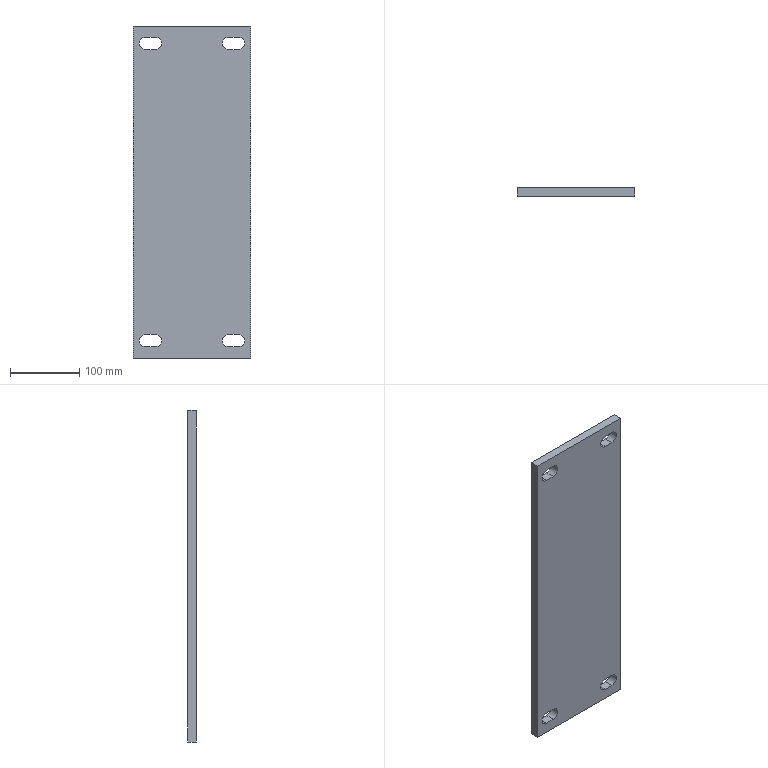Part | SolidWorks | features BaseBody 1 | 1 solid | 22 faces | box 170 x 13 x 480 mm | volume 1034464 mm3 | plane 14 | cylinder 8 | commonest cylinder face diameters 18 x8
STEP:
#1=CARTESIAN_POINT('',(-10.701,8.606,34.));
#2=VERTEX_POINT('',#1);
#3=CARTESIAN_POINT('',(-10.701,8.606,16.));
#4=VERTEX_POINT('',#3);
#5=CARTESIAN_POINT('',(-10.701,8.606,25.));
#6=DIRECTION('',(0.,-1.,0.));
#7=DIRECTION('',(0.,0.,-1.));
#8=AXIS2_PLACEMENT_3D('',#5,#6,#7);
#9=CIRCLE('',#8,9.);
#10=EDGE_CURVE('',#2,#4,#9,.T.);
#11=ORIENTED_EDGE('',*,*,#10,.T.);
#12=CARTESIAN_POINT('',(3.299,8.606,16.));
#13=VERTEX_POINT('',#12);
#14=CARTESIAN_POINT('',(-28.701,8.606,16.));
#15=DIRECTION('',(1.,0.,0.));
#16=VECTOR('',#15,1000.);
#17=LINE('',#14,#16);
#18=EDGE_CURVE('',#4,#13,#17,.T.);
#19=ORIENTED_EDGE('',*,*,#18,.T.);
#20=CARTESIAN_POINT('',(3.299,8.606,34.));
#21=VERTEX_POINT('',#20);
#22=CARTESIAN_POINT('',(3.299,8.606,25.));
#23=DIRECTION('',(0.,-1.,0.));
#24=DIRECTION('',(0.,0.,-1.));
#25=AXIS2_PLACEMENT_3D('',#22,#23,#24);
#26=CIRCLE('',#25,9.);
#27=EDGE_CURVE('',#13,#21,#26,.T.);
#28=ORIENTED_EDGE('',*,*,#27,.T.);
#29=CARTESIAN_POINT('',(-28.701,8.606,34.));
#30=DIRECTION('',(-1.,0.,0.));
#31=VECTOR('',#30,1000.);
#32=LINE('',#29,#31);
#33=EDGE_CURVE('',#21,#2,#32,.T.);
#34=ORIENTED_EDGE('',*,*,#33,.T.);
#35=EDGE_LOOP('',(#11,#19,#28,#34));
#36=FACE_BOUND('',#35,.T.);
#37=CARTESIAN_POINT('',(-10.701,8.606,446.));
#38=VERTEX_POINT('',#37);
#39=CARTESIAN_POINT('',(3.299,8.606,446.));
#40=VERTEX_POINT('',#39);
#41=CARTESIAN_POINT('',(-28.701,8.606,446.));
#42=DIRECTION('',(1.,0.,0.));
#43=VECTOR('',#42,1000.);
#44=LINE('',#41,#43);
#45=EDGE_CURVE('',#38,#40,#44,.T.);
#46=ORIENTED_EDGE('',*,*,#45,.T.);
#47=CARTESIAN_POINT('',(3.299,8.606,464.));
#48=VERTEX_POINT('',#47);
#49=CARTESIAN_POINT('',(3.299,8.606,455.));
#50=DIRECTION('',(0.,-1.,0.));
#51=DIRECTION('',(0.,0.,-1.));
#52=AXIS2_PLACEMENT_3D('',#49,#50,#51);
#53=CIRCLE('',#52,9.);
#54=EDGE_CURVE('',#40,#48,#53,.T.);
#55=ORIENTED_EDGE('',*,*,#54,.T.);
#56=CARTESIAN_POINT('',(-10.701,8.606,464.));
#57=VERTEX_POINT('',#56);
#58=CARTESIAN_POINT('',(-28.701,8.606,464.));
#59=DIRECTION('',(-1.,0.,0.));
#60=VECTOR('',#59,1000.);
#61=LINE('',#58,#60);
#62=EDGE_CURVE('',#48,#57,#61,.T.);
#63=ORIENTED_EDGE('',*,*,#62,.T.);
#64=CARTESIAN_POINT('',(-10.701,8.606,455.));
#65=DIRECTION('',(0.,-1.,0.));
#66=DIRECTION('',(0.,0.,-1.));
#67=AXIS2_PLACEMENT_3D('',#64,#65,#66);
#68=CIRCLE('',#67,9.);
#69=EDGE_CURVE('',#57,#38,#68,.T.);
#70=ORIENTED_EDGE('',*,*,#69,.T.);
#71=EDGE_LOOP('',(#46,#55,#63,#70));
#72=FACE_BOUND('',#71,.T.);
#73=CARTESIAN_POINT('',(109.299,8.606,16.));
#74=VERTEX_POINT('',#73);
#75=CARTESIAN_POINT('',(123.299,8.606,16.));
#76=VERTEX_POINT('',#75);
#77=CARTESIAN_POINT('',(-28.701,8.606,16.));
#78=DIRECTION('',(1.,0.,0.));
#79=VECTOR('',#78,1000.);
#80=LINE('',#77,#79);
#81=EDGE_CURVE('',#74,#76,#80,.T.);
#82=ORIENTED_EDGE('',*,*,#81,.T.);
#83=CARTESIAN_POINT('',(123.299,8.606,34.));
#84=VERTEX_POINT('',#83);
#85=CARTESIAN_POINT('',(123.299,8.606,25.));
#86=DIRECTION('',(0.,-1.,0.));
#87=DIRECTION('',(0.,0.,-1.));
#88=AXIS2_PLACEMENT_3D('',#85,#86,#87);
#89=CIRCLE('',#88,9.);
#90=EDGE_CURVE('',#76,#84,#89,.T.);
#91=ORIENTED_EDGE('',*,*,#90,.T.);
#92=CARTESIAN_POINT('',(109.299,8.606,34.));
#93=VERTEX_POINT('',#92);
#94=CARTESIAN_POINT('',(-28.701,8.606,34.));
#95=DIRECTION('',(-1.,0.,0.));
#96=VECTOR('',#95,1000.);
#97=LINE('',#94,#96);
#98=EDGE_CURVE('',#84,#93,#97,.T.);
#99=ORIENTED_EDGE('',*,*,#98,.T.);
#100=CARTESIAN_POINT('',(109.299,8.606,25.));
#101=DIRECTION('',(0.,-1.,0.));
#102=DIRECTION('',(0.,0.,-1.));
#103=AXIS2_PLACEMENT_3D('',#100,#101,#102);
#104=CIRCLE('',#103,9.);
#105=EDGE_CURVE('',#93,#74,#104,.T.);
#106=ORIENTED_EDGE('',*,*,#105,.T.);
#107=EDGE_LOOP('',(#82,#91,#99,#106));
#108=FACE_BOUND('',#107,.T.);
#109=CARTESIAN_POINT('',(109.299,8.606,446.));
#110=VERTEX_POINT('',#109);
#111=CARTESIAN_POINT('',(123.299,8.606,446.));
#112=VERTEX_POINT('',#111);
#113=CARTESIAN_POINT('',(-28.701,8.606,446.));
#114=DIRECTION('',(1.,0.,0.));
#115=VECTOR('',#114,1000.);
#116=LINE('',#113,#115);
#117=EDGE_CURVE('',#110,#112,#116,.T.);
#118=ORIENTED_EDGE('',*,*,#117,.T.);
#119=CARTESIAN_POINT('',(123.299,8.606,464.));
#120=VERTEX_POINT('',#119);
#121=CARTESIAN_POINT('',(123.299,8.606,455.));
#122=DIRECTION('',(0.,-1.,0.));
#123=DIRECTION('',(0.,0.,-1.));
#124=AXIS2_PLACEMENT_3D('',#121,#122,#123);
#125=CIRCLE('',#124,9.);
#126=EDGE_CURVE('',#112,#120,#125,.T.);
#127=ORIENTED_EDGE('',*,*,#126,.T.);
#128=CARTESIAN_POINT('',(109.299,8.606,464.));
#129=VERTEX_POINT('',#128);
#130=CARTESIAN_POINT('',(-28.701,8.606,464.));
#131=DIRECTION('',(-1.,0.,0.));
#132=VECTOR('',#131,1000.);
#133=LINE('',#130,#132);
#134=EDGE_CURVE('',#120,#129,#133,.T.);
#135=ORIENTED_EDGE('',*,*,#134,.T.);
#136=CARTESIAN_POINT('',(109.299,8.606,455.));
#137=DIRECTION('',(0.,-1.,0.));
#138=DIRECTION('',(0.,0.,-1.));
#139=AXIS2_PLACEMENT_3D('',#136,#137,#138);
#140=CIRCLE('',#139,9.);
#141=EDGE_CURVE('',#129,#110,#140,.T.);
#142=ORIENTED_EDGE('',*,*,#141,.T.);
#143=EDGE_LOOP('',(#118,#127,#135,#142));
#144=FACE_BOUND('',#143,.T.);
#145=CARTESIAN_POINT('',(141.299,8.606,0.));
#146=VERTEX_POINT('',#145);
#147=CARTESIAN_POINT('',(-28.701,8.606,0.));
#148=VERTEX_POINT('',#147);
#149=CARTESIAN_POINT('',(-28.701,8.606,0.));
#150=DIRECTION('',(-1.,0.,0.));
#151=VECTOR('',#150,1000.);
#152=LINE('',#149,#151);
#153=EDGE_CURVE('',#146,#148,#152,.T.);
#154=ORIENTED_EDGE('',*,*,#153,.T.);
#155=CARTESIAN_POINT('',(-28.701,8.606,480.));
#156=VERTEX_POINT('',#155);
#157=CARTESIAN_POINT('',(-28.701,8.606,0.));
#158=DIRECTION('',(0.,0.,1.));
#159=VECTOR('',#158,1000.);
#160=LINE('',#157,#159);
#161=EDGE_CURVE('',#148,#156,#160,.T.);
#162=ORIENTED_EDGE('',*,*,#161,.T.);
#163=CARTESIAN_POINT('',(141.299,8.606,480.));
#164=VERTEX_POINT('',#163);
#165=CARTESIAN_POINT('',(-28.701,8.606,480.));
#166=DIRECTION('',(1.,0.,0.));
#167=VECTOR('',#166,1000.);
#168=LINE('',#165,#167);
#169=EDGE_CURVE('',#156,#164,#168,.T.);
#170=ORIENTED_EDGE('',*,*,#169,.T.);
#171=CARTESIAN_POINT('',(141.299,8.606,0.));
#172=DIRECTION('',(0.,0.,-1.));
#173=VECTOR('',#172,1000.);
#174=LINE('',#171,#173);
#175=EDGE_CURVE('',#164,#146,#174,.T.);
#176=ORIENTED_EDGE('',*,*,#175,.T.);
#177=EDGE_LOOP('',(#154,#162,#170,#176));
#178=FACE_OUTER_BOUND('',#177,.T.);
#179=CARTESIAN_POINT('',(-28.701,8.606,0.));
#180=DIRECTION('',(0.,1.,0.));
#181=DIRECTION('',(0.,0.,1.));
#182=AXIS2_PLACEMENT_3D('',#179,#180,#181);
#183=PLANE('',#182);
#184=ADVANCED_FACE('',(#36,#72,#108,#144,#178),#183,.T.);
#185=CARTESIAN_POINT('',(3.299,-4.394,16.));
#186=VERTEX_POINT('',#185);
#187=CARTESIAN_POINT('',(3.299,8.606,16.));
#188=DIRECTION('',(0.,-1.,0.));
#189=VECTOR('',#188,1000.);
#190=LINE('',#187,#189);
#191=EDGE_CURVE('',#13,#186,#190,.T.);
#192=ORIENTED_EDGE('',*,*,#191,.F.);
#193=ORIENTED_EDGE('',*,*,#18,.F.);
#194=CARTESIAN_POINT('',(-10.701,-4.394,16.));
#195=VERTEX_POINT('',#194);
#196=CARTESIAN_POINT('',(-10.701,8.606,16.));
#197=DIRECTION('',(0.,1.,0.));
#198=VECTOR('',#197,1000.);
#199=LINE('',#196,#198);
#200=EDGE_CURVE('',#195,#4,#199,.T.);
#201=ORIENTED_EDGE('',*,*,#200,.F.);
#202=CARTESIAN_POINT('',(3.299,-4.394,16.));
#203=DIRECTION('',(-1.,0.,0.));
#204=VECTOR('',#203,1000.);
#205=LINE('',#202,#204);
#206=EDGE_CURVE('',#186,#195,#205,.T.);
#207=ORIENTED_EDGE('',*,*,#206,.F.);
#208=EDGE_LOOP('',(#192,#193,#201,#207));
#209=FACE_OUTER_BOUND('',#208,.T.);
#210=CARTESIAN_POINT('',(3.299,8.606,16.));
#211=DIRECTION('',(0.,0.,-1.));
#212=DIRECTION('',(-1.,0.,0.));
#213=AXIS2_PLACEMENT_3D('',#210,#211,#212);
#214=PLANE('',#213);
#215=ADVANCED_FACE('',(#209),#214,.F.);
#216=ORIENTED_EDGE('',*,*,#200,.T.);
#217=ORIENTED_EDGE('',*,*,#10,.F.);
#218=CARTESIAN_POINT('',(-10.701,-4.394,34.));
#219=VERTEX_POINT('',#218);
#220=CARTESIAN_POINT('',(-10.701,8.606,34.));
#221=DIRECTION('',(0.,1.,0.));
#222=VECTOR('',#221,1000.);
#223=LINE('',#220,#222);
#224=EDGE_CURVE('',#219,#2,#223,.T.);
#225=ORIENTED_EDGE('',*,*,#224,.F.);
#226=CARTESIAN_POINT('',(-10.701,-4.394,25.));
#227=DIRECTION('',(0.,1.,0.));
#228=DIRECTION('',(0.,0.,-1.));
#229=AXIS2_PLACEMENT_3D('',#226,#227,#228);
#230=CIRCLE('',#229,9.);
#231=EDGE_CURVE('',#195,#219,#230,.T.);
#232=ORIENTED_EDGE('',*,*,#231,.F.);
#233=EDGE_LOOP('',(#216,#217,#225,#232));
#234=FACE_OUTER_BOUND('',#233,.T.);
#235=CARTESIAN_POINT('',(-10.701,8.606,25.));
#236=DIRECTION('',(0.,-1.,0.));
#237=DIRECTION('',(0.,0.,-1.));
#238=AXIS2_PLACEMENT_3D('',#235,#236,#237);
#239=CYLINDRICAL_SURFACE('',#238,9.);
#240=ADVANCED_FACE('',(#234),#239,.F.);
#241=ORIENTED_EDGE('',*,*,#224,.T.);
#242=ORIENTED_EDGE('',*,*,#33,.F.);
#243=CARTESIAN_POINT('',(3.299,-4.394,34.));
#244=VERTEX_POINT('',#243);
#245=CARTESIAN_POINT('',(3.299,8.606,34.));
#246=DIRECTION('',(0.,1.,0.));
#247=VECTOR('',#246,1000.);
#248=LINE('',#245,#247);
#249=EDGE_CURVE('',#244,#21,#248,.T.);
#250=ORIENTED_EDGE('',*,*,#249,.F.);
#251=CARTESIAN_POINT('',(-10.701,-4.394,34.));
#252=DIRECTION('',(1.,0.,0.));
#253=VECTOR('',#252,1000.);
#254=LINE('',#251,#253);
#255=EDGE_CURVE('',#219,#244,#254,.T.);
#256=ORIENTED_EDGE('',*,*,#255,.F.);
#257=EDGE_LOOP('',(#241,#242,#250,#256));
#258=FACE_OUTER_BOUND('',#257,.T.);
#259=CARTESIAN_POINT('',(-10.701,8.606,34.));
#260=DIRECTION('',(0.,0.,1.));
#261=DIRECTION('',(1.,0.,0.));
#262=AXIS2_PLACEMENT_3D('',#259,#260,#261);
#263=PLANE('',#262);
#264=ADVANCED_FACE('',(#258),#263,.F.);
#265=ORIENTED_EDGE('',*,*,#249,.T.);
#266=ORIENTED_EDGE('',*,*,#27,.F.);
#267=ORIENTED_EDGE('',*,*,#191,.T.);
#268=CARTESIAN_POINT('',(3.299,-4.394,25.));
#269=DIRECTION('',(0.,1.,0.));
#270=DIRECTION('',(0.,0.,-1.));
#271=AXIS2_PLACEMENT_3D('',#268,#269,#270);
#272=CIRCLE('',#271,9.);
#273=EDGE_CURVE('',#244,#186,#272,.T.);
#274=ORIENTED_EDGE('',*,*,#273,.F.);
#275=EDGE_LOOP('',(#265,#266,#267,#274));
#276=FACE_OUTER_BOUND('',#275,.T.);
#277=CARTESIAN_POINT('',(3.299,8.606,25.));
#278=DIRECTION('',(0.,-1.,0.));
#279=DIRECTION('',(0.,0.,-1.));
#280=AXIS2_PLACEMENT_3D('',#277,#278,#279);
#281=CYLINDRICAL_SURFACE('',#280,9.);
#282=ADVANCED_FACE('',(#276),#281,.F.);
#283=CARTESIAN_POINT('',(3.299,-4.394,464.));
#284=VERTEX_POINT('',#283);
#285=CARTESIAN_POINT('',(3.299,8.606,464.));
#286=DIRECTION('',(0.,-1.,0.));
#287=VECTOR('',#286,1000.);
#288=LINE('',#285,#287);
#289=EDGE_CURVE('',#48,#284,#288,.T.);
#290=ORIENTED_EDGE('',*,*,#289,.F.);
#291=ORIENTED_EDGE('',*,*,#54,.F.);
#292=CARTESIAN_POINT('',(3.299,-4.394,446.));
#293=VERTEX_POINT('',#292);
#294=CARTESIAN_POINT('',(3.299,8.606,446.));
#295=DIRECTION('',(0.,1.,0.));
#296=VECTOR('',#295,1000.);
#297=LINE('',#294,#296);
#298=EDGE_CURVE('',#293,#40,#297,.T.);
#299=ORIENTED_EDGE('',*,*,#298,.F.);
#300=CARTESIAN_POINT('',(3.299,-4.394,455.));
#301=DIRECTION('',(0.,1.,0.));
#302=DIRECTION('',(0.,0.,-1.));
#303=AXIS2_PLACEMENT_3D('',#300,#301,#302);
#304=CIRCLE('',#303,9.);
#305=EDGE_CURVE('',#284,#293,#304,.T.);
#306=ORIENTED_EDGE('',*,*,#305,.F.);
#307=EDGE_LOOP('',(#290,#291,#299,#306));
#308=FACE_OUTER_BOUND('',#307,.T.);
#309=CARTESIAN_POINT('',(3.299,8.606,455.));
#310=DIRECTION('',(0.,-1.,0.));
#311=DIRECTION('',(0.,0.,-1.));
#312=AXIS2_PLACEMENT_3D('',#309,#310,#311);
#313=CYLINDRICAL_SURFACE('',#312,9.);
#314=ADVANCED_FACE('',(#308),#313,.F.);
#315=ORIENTED_EDGE('',*,*,#298,.T.);
#316=ORIENTED_EDGE('',*,*,#45,.F.);
#317=CARTESIAN_POINT('',(-10.701,-4.394,446.));
#318=VERTEX_POINT('',#317);
#319=CARTESIAN_POINT('',(-10.701,8.606,446.));
#320=DIRECTION('',(0.,1.,0.));
#321=VECTOR('',#320,1000.);
#322=LINE('',#319,#321);
#323=EDGE_CURVE('',#318,#38,#322,.T.);
#324=ORIENTED_EDGE('',*,*,#323,.F.);
#325=CARTESIAN_POINT('',(3.299,-4.394,446.));
#326=DIRECTION('',(-1.,0.,0.));
#327=VECTOR('',#326,1000.);
#328=LINE('',#325,#327);
#329=EDGE_CURVE('',#293,#318,#328,.T.);
#330=ORIENTED_EDGE('',*,*,#329,.F.);
#331=EDGE_LOOP('',(#315,#316,#324,#330));
#332=FACE_OUTER_BOUND('',#331,.T.);
#333=CARTESIAN_POINT('',(3.299,8.606,446.));
#334=DIRECTION('',(0.,0.,-1.));
#335=DIRECTION('',(-1.,0.,0.));
#336=AXIS2_PLACEMENT_3D('',#333,#334,#335);
#337=PLANE('',#336);
#338=ADVANCED_FACE('',(#332),#337,.F.);
#339=ORIENTED_EDGE('',*,*,#323,.T.);
#340=ORIENTED_EDGE('',*,*,#69,.F.);
#341=CARTESIAN_POINT('',(-10.701,-4.394,464.));
#342=VERTEX_POINT('',#341);
#343=CARTESIAN_POINT('',(-10.701,8.606,464.));
#344=DIRECTION('',(0.,1.,0.));
#345=VECTOR('',#344,1000.);
#346=LINE('',#343,#345);
#347=EDGE_CURVE('',#342,#57,#346,.T.);
#348=ORIENTED_EDGE('',*,*,#347,.F.);
#349=CARTESIAN_POINT('',(-10.701,-4.394,455.));
#350=DIRECTION('',(0.,1.,0.));
#351=DIRECTION('',(0.,0.,-1.));
#352=AXIS2_PLACEMENT_3D('',#349,#350,#351);
#353=CIRCLE('',#352,9.);
#354=EDGE_CURVE('',#318,#342,#353,.T.);
#355=ORIENTED_EDGE('',*,*,#354,.F.);
#356=EDGE_LOOP('',(#339,#340,#348,#355));
#357=FACE_OUTER_BOUND('',#356,.T.);
#358=CARTESIAN_POINT('',(-10.701,8.606,455.));
#359=DIRECTION('',(0.,-1.,0.));
#360=DIRECTION('',(0.,0.,-1.));
#361=AXIS2_PLACEMENT_3D('',#358,#359,#360);
#362=CYLINDRICAL_SURFACE('',#361,9.);
#363=ADVANCED_FACE('',(#357),#362,.F.);
#364=ORIENTED_EDGE('',*,*,#347,.T.);
#365=ORIENTED_EDGE('',*,*,#62,.F.);
#366=ORIENTED_EDGE('',*,*,#289,.T.);
#367=CARTESIAN_POINT('',(-10.701,-4.394,464.));
#368=DIRECTION('',(1.,0.,0.));
#369=VECTOR('',#368,1000.);
#370=LINE('',#367,#369);
#371=EDGE_CURVE('',#342,#284,#370,.T.);
#372=ORIENTED_EDGE('',*,*,#371,.F.);
#373=EDGE_LOOP('',(#364,#365,#366,#372));
#374=FACE_OUTER_BOUND('',#373,.T.);
#375=CARTESIAN_POINT('',(-10.701,8.606,464.));
#376=DIRECTION('',(0.,0.,1.));
#377=DIRECTION('',(1.,0.,0.));
#378=AXIS2_PLACEMENT_3D('',#375,#376,#377);
#379=PLANE('',#378);
#380=ADVANCED_FACE('',(#374),#379,.F.);
#381=CARTESIAN_POINT('',(123.299,-4.394,34.));
#382=VERTEX_POINT('',#381);
#383=CARTESIAN_POINT('',(123.299,8.606,34.));
#384=DIRECTION('',(0.,-1.,0.));
#385=VECTOR('',#384,1000.);
#386=LINE('',#383,#385);
#387=EDGE_CURVE('',#84,#382,#386,.T.);
#388=ORIENTED_EDGE('',*,*,#387,.F.);
#389=ORIENTED_EDGE('',*,*,#90,.F.);
#390=CARTESIAN_POINT('',(123.299,-4.394,16.));
#391=VERTEX_POINT('',#390);
#392=CARTESIAN_POINT('',(123.299,8.606,16.));
#393=DIRECTION('',(0.,1.,0.));
#394=VECTOR('',#393,1000.);
#395=LINE('',#392,#394);
#396=EDGE_CURVE('',#391,#76,#395,.T.);
#397=ORIENTED_EDGE('',*,*,#396,.F.);
#398=CARTESIAN_POINT('',(123.299,-4.394,25.));
#399=DIRECTION('',(0.,1.,0.));
#400=DIRECTION('',(0.,0.,-1.));
#401=AXIS2_PLACEMENT_3D('',#398,#399,#400);
#402=CIRCLE('',#401,9.);
#403=EDGE_CURVE('',#382,#391,#402,.T.);
#404=ORIENTED_EDGE('',*,*,#403,.F.);
#405=EDGE_LOOP('',(#388,#389,#397,#404));
#406=FACE_OUTER_BOUND('',#405,.T.);
#407=CARTESIAN_POINT('',(123.299,8.606,25.));
#408=DIRECTION('',(0.,-1.,0.));
#409=DIRECTION('',(0.,0.,-1.));
#410=AXIS2_PLACEMENT_3D('',#407,#408,#409);
#411=CYLINDRICAL_SURFACE('',#410,9.);
#412=ADVANCED_FACE('',(#406),#411,.F.);
#413=ORIENTED_EDGE('',*,*,#396,.T.);
#414=ORIENTED_EDGE('',*,*,#81,.F.);
#415=CARTESIAN_POINT('',(109.299,-4.394,16.));
#416=VERTEX_POINT('',#415);
#417=CARTESIAN_POINT('',(109.299,8.606,16.));
#418=DIRECTION('',(0.,1.,0.));
#419=VECTOR('',#418,1000.);
#420=LINE('',#417,#419);
#421=EDGE_CURVE('',#416,#74,#420,.T.);
#422=ORIENTED_EDGE('',*,*,#421,.F.);
#423=CARTESIAN_POINT('',(123.299,-4.394,16.));
#424=DIRECTION('',(-1.,0.,0.));
#425=VECTOR('',#424,1000.);
#426=LINE('',#423,#425);
#427=EDGE_CURVE('',#391,#416,#426,.T.);
#428=ORIENTED_EDGE('',*,*,#427,.F.);
#429=EDGE_LOOP('',(#413,#414,#422,#428));
#430=FACE_OUTER_BOUND('',#429,.T.);
#431=CARTESIAN_POINT('',(123.299,8.606,16.));
#432=DIRECTION('',(0.,0.,-1.));
#433=DIRECTION('',(-1.,0.,0.));
#434=AXIS2_PLACEMENT_3D('',#431,#432,#433);
#435=PLANE('',#434);
#436=ADVANCED_FACE('',(#430),#435,.F.);
#437=ORIENTED_EDGE('',*,*,#421,.T.);
#438=ORIENTED_EDGE('',*,*,#105,.F.);
#439=CARTESIAN_POINT('',(109.299,-4.394,34.));
#440=VERTEX_POINT('',#439);
#441=CARTESIAN_POINT('',(109.299,8.606,34.));
#442=DIRECTION('',(0.,1.,0.));
#443=VECTOR('',#442,1000.);
#444=LINE('',#441,#443);
#445=EDGE_CURVE('',#440,#93,#444,.T.);
#446=ORIENTED_EDGE('',*,*,#445,.F.);
#447=CARTESIAN_POINT('',(109.299,-4.394,25.));
#448=DIRECTION('',(0.,1.,0.));
#449=DIRECTION('',(0.,0.,-1.));
#450=AXIS2_PLACEMENT_3D('',#447,#448,#449);
#451=CIRCLE('',#450,9.);
#452=EDGE_CURVE('',#416,#440,#451,.T.);
#453=ORIENTED_EDGE('',*,*,#452,.F.);
#454=EDGE_LOOP('',(#437,#438,#446,#453));
#455=FACE_OUTER_BOUND('',#454,.T.);
#456=CARTESIAN_POINT('',(109.299,8.606,25.));
#457=DIRECTION('',(0.,-1.,0.));
#458=DIRECTION('',(0.,0.,-1.));
#459=AXIS2_PLACEMENT_3D('',#456,#457,#458);
#460=CYLINDRICAL_SURFACE('',#459,9.);
#461=ADVANCED_FACE('',(#455),#460,.F.);
#462=ORIENTED_EDGE('',*,*,#445,.T.);
#463=ORIENTED_EDGE('',*,*,#98,.F.);
#464=ORIENTED_EDGE('',*,*,#387,.T.);
#465=CARTESIAN_POINT('',(109.299,-4.394,34.));
#466=DIRECTION('',(1.,0.,0.));
#467=VECTOR('',#466,1000.);
#468=LINE('',#465,#467);
#469=EDGE_CURVE('',#440,#382,#468,.T.);
#470=ORIENTED_EDGE('',*,*,#469,.F.);
#471=EDGE_LOOP('',(#462,#463,#464,#470));
#472=FACE_OUTER_BOUND('',#471,.T.);
#473=CARTESIAN_POINT('',(109.299,8.606,34.));
#474=DIRECTION('',(0.,0.,1.));
#475=DIRECTION('',(1.,0.,0.));
#476=AXIS2_PLACEMENT_3D('',#473,#474,#475);
#477=PLANE('',#476);
#478=ADVANCED_FACE('',(#472),#477,.F.);
#479=CARTESIAN_POINT('',(123.299,-4.394,464.));
#480=VERTEX_POINT('',#479);
#481=CARTESIAN_POINT('',(123.299,8.606,464.));
#482=DIRECTION('',(0.,-1.,0.));
#483=VECTOR('',#482,1000.);
#484=LINE('',#481,#483);
#485=EDGE_CURVE('',#120,#480,#484,.T.);
#486=ORIENTED_EDGE('',*,*,#485,.F.);
#487=ORIENTED_EDGE('',*,*,#126,.F.);
#488=CARTESIAN_POINT('',(123.299,-4.394,446.));
#489=VERTEX_POINT('',#488);
#490=CARTESIAN_POINT('',(123.299,8.606,446.));
#491=DIRECTION('',(0.,1.,0.));
#492=VECTOR('',#491,1000.);
#493=LINE('',#490,#492);
#494=EDGE_CURVE('',#489,#112,#493,.T.);
#495=ORIENTED_EDGE('',*,*,#494,.F.);
#496=CARTESIAN_POINT('',(123.299,-4.394,455.));
#497=DIRECTION('',(0.,1.,0.));
#498=DIRECTION('',(0.,0.,-1.));
#499=AXIS2_PLACEMENT_3D('',#496,#497,#498);
#500=CIRCLE('',#499,9.);
#501=EDGE_CURVE('',#480,#489,#500,.T.);
#502=ORIENTED_EDGE('',*,*,#501,.F.);
#503=EDGE_LOOP('',(#486,#487,#495,#502));
#504=FACE_OUTER_BOUND('',#503,.T.);
#505=CARTESIAN_POINT('',(123.299,8.606,455.));
#506=DIRECTION('',(0.,-1.,0.));
#507=DIRECTION('',(0.,0.,-1.));
#508=AXIS2_PLACEMENT_3D('',#505,#506,#507);
#509=CYLINDRICAL_SURFACE('',#508,9.);
#510=ADVANCED_FACE('',(#504),#509,.F.);
#511=ORIENTED_EDGE('',*,*,#494,.T.);
#512=ORIENTED_EDGE('',*,*,#117,.F.);
#513=CARTESIAN_POINT('',(109.299,-4.394,446.));
#514=VERTEX_POINT('',#513);
#515=CARTESIAN_POINT('',(109.299,8.606,446.));
#516=DIRECTION('',(0.,1.,0.));
#517=VECTOR('',#516,1000.);
#518=LINE('',#515,#517);
#519=EDGE_CURVE('',#514,#110,#518,.T.);
#520=ORIENTED_EDGE('',*,*,#519,.F.);
#521=CARTESIAN_POINT('',(123.299,-4.394,446.));
#522=DIRECTION('',(-1.,0.,0.));
#523=VECTOR('',#522,1000.);
#524=LINE('',#521,#523);
#525=EDGE_CURVE('',#489,#514,#524,.T.);
#526=ORIENTED_EDGE('',*,*,#525,.F.);
#527=EDGE_LOOP('',(#511,#512,#520,#526));
#528=FACE_OUTER_BOUND('',#527,.T.);
#529=CARTESIAN_POINT('',(123.299,8.606,446.));
#530=DIRECTION('',(0.,0.,-1.));
#531=DIRECTION('',(-1.,0.,0.));
#532=AXIS2_PLACEMENT_3D('',#529,#530,#531);
#533=PLANE('',#532);
#534=ADVANCED_FACE('',(#528),#533,.F.);
#535=ORIENTED_EDGE('',*,*,#519,.T.);
#536=ORIENTED_EDGE('',*,*,#141,.F.);
#537=CARTESIAN_POINT('',(109.299,-4.394,464.));
#538=VERTEX_POINT('',#537);
#539=CARTESIAN_POINT('',(109.299,8.606,464.));
#540=DIRECTION('',(0.,1.,0.));
#541=VECTOR('',#540,1000.);
#542=LINE('',#539,#541);
#543=EDGE_CURVE('',#538,#129,#542,.T.);
#544=ORIENTED_EDGE('',*,*,#543,.F.);
#545=CARTESIAN_POINT('',(109.299,-4.394,455.));
#546=DIRECTION('',(0.,1.,0.));
#547=DIRECTION('',(0.,0.,-1.));
#548=AXIS2_PLACEMENT_3D('',#545,#546,#547);
#549=CIRCLE('',#548,9.);
#550=EDGE_CURVE('',#514,#538,#549,.T.);
#551=ORIENTED_EDGE('',*,*,#550,.F.);
#552=EDGE_LOOP('',(#535,#536,#544,#551));
#553=FACE_OUTER_BOUND('',#552,.T.);
#554=CARTESIAN_POINT('',(109.299,8.606,455.));
#555=DIRECTION('',(0.,-1.,0.));
#556=DIRECTION('',(0.,0.,-1.));
#557=AXIS2_PLACEMENT_3D('',#554,#555,#556);
#558=CYLINDRICAL_SURFACE('',#557,9.);
#559=ADVANCED_FACE('',(#553),#558,.F.);
#560=ORIENTED_EDGE('',*,*,#543,.T.);
#561=ORIENTED_EDGE('',*,*,#134,.F.);
#562=ORIENTED_EDGE('',*,*,#485,.T.);
#563=CARTESIAN_POINT('',(109.299,-4.394,464.));
#564=DIRECTION('',(1.,0.,0.));
#565=VECTOR('',#564,1000.);
#566=LINE('',#563,#565);
#567=EDGE_CURVE('',#538,#480,#566,.T.);
#568=ORIENTED_EDGE('',*,*,#567,.F.);
#569=EDGE_LOOP('',(#560,#561,#562,#568));
#570=FACE_OUTER_BOUND('',#569,.T.);
#571=CARTESIAN_POINT('',(109.299,8.606,464.));
#572=DIRECTION('',(0.,0.,1.));
#573=DIRECTION('',(1.,0.,0.));
#574=AXIS2_PLACEMENT_3D('',#571,#572,#573);
#575=PLANE('',#574);
#576=ADVANCED_FACE('',(#570),#575,.F.);
#577=CARTESIAN_POINT('',(-28.701,-4.394,0.));
#578=VERTEX_POINT('',#577);
#579=CARTESIAN_POINT('',(-28.701,-4.394,0.));
#580=DIRECTION('',(0.,-1.,0.));
#581=VECTOR('',#580,1000.);
#582=LINE('',#579,#581);
#583=EDGE_CURVE('',#148,#578,#582,.T.);
#584=ORIENTED_EDGE('',*,*,#583,.T.);
#585=CARTESIAN_POINT('',(-28.701,-4.394,480.));
#586=VERTEX_POINT('',#585);
#587=CARTESIAN_POINT('',(-28.701,-4.394,0.));
#588=DIRECTION('',(0.,0.,1.));
#589=VECTOR('',#588,1000.);
#590=LINE('',#587,#589);
#591=EDGE_CURVE('',#578,#586,#590,.T.);
#592=ORIENTED_EDGE('',*,*,#591,.T.);
#593=CARTESIAN_POINT('',(-28.701,-4.394,480.));
#594=DIRECTION('',(0.,1.,0.));
#595=VECTOR('',#594,1000.);
#596=LINE('',#593,#595);
#597=EDGE_CURVE('',#586,#156,#596,.T.);
#598=ORIENTED_EDGE('',*,*,#597,.T.);
#599=ORIENTED_EDGE('',*,*,#161,.F.);
#600=EDGE_LOOP('',(#584,#592,#598,#599));
#601=FACE_OUTER_BOUND('',#600,.T.);
#602=CARTESIAN_POINT('',(-28.701,-4.394,0.));
#603=DIRECTION('',(-1.,0.,0.));
#604=DIRECTION('',(0.,0.,1.));
#605=AXIS2_PLACEMENT_3D('',#602,#603,#604);
#606=PLANE('',#605);
#607=ADVANCED_FACE('',(#601),#606,.T.);
#608=ORIENTED_EDGE('',*,*,#153,.F.);
#609=CARTESIAN_POINT('',(141.299,-4.394,0.));
#610=VERTEX_POINT('',#609);
#611=CARTESIAN_POINT('',(141.299,2.106,0.));
#612=DIRECTION('',(0.,1.,0.));
#613=VECTOR('',#612,1000.);
#614=LINE('',#611,#613);
#615=EDGE_CURVE('',#610,#146,#614,.T.);
#616=ORIENTED_EDGE('',*,*,#615,.F.);
#617=CARTESIAN_POINT('',(56.299,-4.394,0.));
#618=DIRECTION('',(1.,0.,0.));
#619=VECTOR('',#618,1000.);
#620=LINE('',#617,#619);
#621=EDGE_CURVE('',#578,#610,#620,.T.);
#622=ORIENTED_EDGE('',*,*,#621,.F.);
#623=ORIENTED_EDGE('',*,*,#583,.F.);
#624=EDGE_LOOP('',(#608,#616,#622,#623));
#625=FACE_OUTER_BOUND('',#624,.T.);
#626=CARTESIAN_POINT('',(56.299,2.106,0.));
#627=DIRECTION('',(0.,0.,1.));
#628=DIRECTION('',(1.,0.,0.));
#629=AXIS2_PLACEMENT_3D('',#626,#627,#628);
#630=PLANE('',#629);
#631=ADVANCED_FACE('',(#625),#630,.F.);
#632=ORIENTED_EDGE('',*,*,#615,.T.);
#633=ORIENTED_EDGE('',*,*,#175,.F.);
#634=CARTESIAN_POINT('',(141.299,-4.394,480.));
#635=VERTEX_POINT('',#634);
#636=CARTESIAN_POINT('',(141.299,8.606,480.));
#637=DIRECTION('',(0.,-1.,0.));
#638=VECTOR('',#637,1000.);
#639=LINE('',#636,#638);
#640=EDGE_CURVE('',#164,#635,#639,.T.);
#641=ORIENTED_EDGE('',*,*,#640,.T.);
#642=CARTESIAN_POINT('',(141.299,-4.394,0.));
#643=DIRECTION('',(0.,0.,-1.));
#644=VECTOR('',#643,1000.);
#645=LINE('',#642,#644);
#646=EDGE_CURVE('',#635,#610,#645,.T.);
#647=ORIENTED_EDGE('',*,*,#646,.T.);
#648=EDGE_LOOP('',(#632,#633,#641,#647));
#649=FACE_OUTER_BOUND('',#648,.T.);
#650=CARTESIAN_POINT('',(141.299,8.606,0.));
#651=DIRECTION('',(1.,0.,0.));
#652=DIRECTION('',(0.,0.,-1.));
#653=AXIS2_PLACEMENT_3D('',#650,#651,#652);
#654=PLANE('',#653);
#655=ADVANCED_FACE('',(#649),#654,.T.);
#656=CARTESIAN_POINT('',(56.299,-4.394,480.));
#657=DIRECTION('',(1.,0.,0.));
#658=VECTOR('',#657,1000.);
#659=LINE('',#656,#658);
#660=EDGE_CURVE('',#586,#635,#659,.T.);
#661=ORIENTED_EDGE('',*,*,#660,.T.);
#662=ORIENTED_EDGE('',*,*,#640,.F.);
#663=ORIENTED_EDGE('',*,*,#169,.F.);
#664=ORIENTED_EDGE('',*,*,#597,.F.);
#665=EDGE_LOOP('',(#661,#662,#663,#664));
#666=FACE_OUTER_BOUND('',#665,.T.);
#667=CARTESIAN_POINT('',(56.299,2.106,480.));
#668=DIRECTION('',(0.,0.,1.));
#669=DIRECTION('',(1.,0.,0.));
#670=AXIS2_PLACEMENT_3D('',#667,#668,#669);
#671=PLANE('',#670);
#672=ADVANCED_FACE('',(#666),#671,.T.);
#673=ORIENTED_EDGE('',*,*,#231,.T.);
#674=ORIENTED_EDGE('',*,*,#255,.T.);
#675=ORIENTED_EDGE('',*,*,#273,.T.);
#676=ORIENTED_EDGE('',*,*,#206,.T.);
#677=EDGE_LOOP('',(#673,#674,#675,#676));
#678=FACE_BOUND('',#677,.T.);
#679=ORIENTED_EDGE('',*,*,#329,.T.);
#680=ORIENTED_EDGE('',*,*,#354,.T.);
#681=ORIENTED_EDGE('',*,*,#371,.T.);
#682=ORIENTED_EDGE('',*,*,#305,.T.);
#683=EDGE_LOOP('',(#679,#680,#681,#682));
#684=FACE_BOUND('',#683,.T.);
#685=ORIENTED_EDGE('',*,*,#427,.T.);
#686=ORIENTED_EDGE('',*,*,#452,.T.);
#687=ORIENTED_EDGE('',*,*,#469,.T.);
#688=ORIENTED_EDGE('',*,*,#403,.T.);
#689=EDGE_LOOP('',(#685,#686,#687,#688));
#690=FACE_BOUND('',#689,.T.);
#691=ORIENTED_EDGE('',*,*,#525,.T.);
#692=ORIENTED_EDGE('',*,*,#550,.T.);
#693=ORIENTED_EDGE('',*,*,#567,.T.);
#694=ORIENTED_EDGE('',*,*,#501,.T.);
#695=EDGE_LOOP('',(#691,#692,#693,#694));
#696=FACE_BOUND('',#695,.T.);
#697=ORIENTED_EDGE('',*,*,#621,.T.);
#698=ORIENTED_EDGE('',*,*,#646,.F.);
#699=ORIENTED_EDGE('',*,*,#660,.F.);
#700=ORIENTED_EDGE('',*,*,#591,.F.);
#701=EDGE_LOOP('',(#697,#698,#699,#700));
#702=FACE_OUTER_BOUND('',#701,.T.);
#703=CARTESIAN_POINT('',(141.299,-4.394,0.));
#704=DIRECTION('',(0.,-1.,0.));
#705=DIRECTION('',(0.,0.,-1.));
#706=AXIS2_PLACEMENT_3D('',#703,#704,#705);
#707=PLANE('',#706);
#708=ADVANCED_FACE('',(#678,#684,#690,#696,#702),#707,.T.);
#709=CLOSED_SHELL('',(#184,#215,#240,#264,#282,#314,#338,#363,#380,#412,#436,#461,#478,#510,#534,#559,#576,#607,#631,#655,#672,#708));
#710=MANIFOLD_SOLID_BREP('',#709);
#711=CARTESIAN_POINT('',(0.,0.,0.));
#712=DIRECTION('',(0.,0.,1.));
#713=DIRECTION('',(1.,0.,0.));
#714=AXIS2_PLACEMENT_3D('',#711,#712,#713);
#715=(LENGTH_UNIT()NAMED_UNIT(*)SI_UNIT(.MILLI.,.METRE.));
#716=UNCERTAINTY_MEASURE_WITH_UNIT(LENGTH_MEASURE(0.00001),#715,'','');
#717=(NAMED_UNIT(*)PLANE_ANGLE_UNIT()SI_UNIT($,.RADIAN.));
#718=(NAMED_UNIT(*)SI_UNIT($,.STERADIAN.)SOLID_ANGLE_UNIT());
#719=(GEOMETRIC_REPRESENTATION_CONTEXT(3)GLOBAL_UNCERTAINTY_ASSIGNED_CONTEXT((#716))GLOBAL_UNIT_ASSIGNED_CONTEXT((#715,#717,#718))REPRESENTATION_CONTEXT('',''));
#720=ADVANCED_BREP_SHAPE_REPRESENTATION('',(#710,#714),#719);